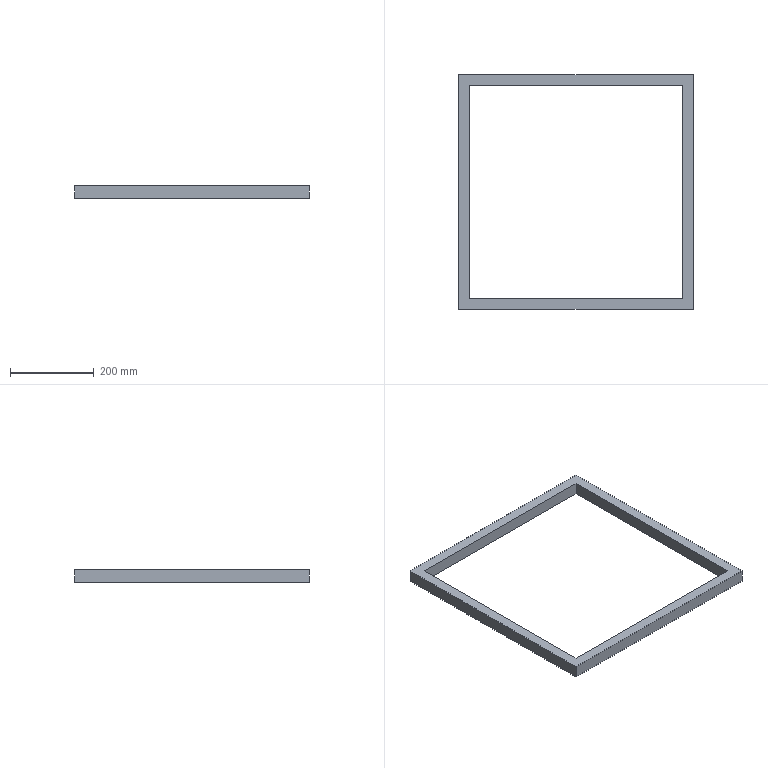Part | SolidWorks | features Extrusion 1 | 1 solid | 10 faces | box 560 x 560 x 30 mm | volume 1605000 mm3 | plane 10
STEP:
#1=CARTESIAN_POINT('',(0.,560.,30.));
#2=VERTEX_POINT('',#1);
#3=CARTESIAN_POINT('',(0.,0.,30.));
#4=VERTEX_POINT('',#3);
#5=CARTESIAN_POINT('',(0.,0.,30.));
#6=DIRECTION('',(0.,-1.,0.));
#7=VECTOR('',#6,1000.);
#8=LINE('',#5,#7);
#9=EDGE_CURVE('',#2,#4,#8,.T.);
#10=ORIENTED_EDGE('',*,*,#9,.T.);
#11=CARTESIAN_POINT('',(560.,0.,30.));
#12=VERTEX_POINT('',#11);
#13=CARTESIAN_POINT('',(0.,0.,30.));
#14=DIRECTION('',(1.,0.,0.));
#15=VECTOR('',#14,1000.);
#16=LINE('',#13,#15);
#17=EDGE_CURVE('',#4,#12,#16,.T.);
#18=ORIENTED_EDGE('',*,*,#17,.T.);
#19=CARTESIAN_POINT('',(560.,560.,30.));
#20=VERTEX_POINT('',#19);
#21=CARTESIAN_POINT('',(560.,0.,30.));
#22=DIRECTION('',(0.,1.,0.));
#23=VECTOR('',#22,1000.);
#24=LINE('',#21,#23);
#25=EDGE_CURVE('',#12,#20,#24,.T.);
#26=ORIENTED_EDGE('',*,*,#25,.T.);
#27=CARTESIAN_POINT('',(0.,560.,30.));
#28=DIRECTION('',(-1.,0.,0.));
#29=VECTOR('',#28,1000.);
#30=LINE('',#27,#29);
#31=EDGE_CURVE('',#20,#2,#30,.T.);
#32=ORIENTED_EDGE('',*,*,#31,.T.);
#33=EDGE_LOOP('',(#10,#18,#26,#32));
#34=FACE_OUTER_BOUND('',#33,.T.);
#35=CARTESIAN_POINT('',(25.,535.,30.));
#36=VERTEX_POINT('',#35);
#37=CARTESIAN_POINT('',(25.,25.,30.));
#38=VERTEX_POINT('',#37);
#39=CARTESIAN_POINT('',(25.,25.,30.));
#40=DIRECTION('',(0.,-1.,0.));
#41=VECTOR('',#40,1000.);
#42=LINE('',#39,#41);
#43=EDGE_CURVE('',#36,#38,#42,.T.);
#44=ORIENTED_EDGE('',*,*,#43,.F.);
#45=CARTESIAN_POINT('',(535.,535.,30.));
#46=VERTEX_POINT('',#45);
#47=CARTESIAN_POINT('',(25.,535.,30.));
#48=DIRECTION('',(-1.,0.,0.));
#49=VECTOR('',#48,1000.);
#50=LINE('',#47,#49);
#51=EDGE_CURVE('',#46,#36,#50,.T.);
#52=ORIENTED_EDGE('',*,*,#51,.F.);
#53=CARTESIAN_POINT('',(535.,25.,30.));
#54=VERTEX_POINT('',#53);
#55=CARTESIAN_POINT('',(535.,25.,30.));
#56=DIRECTION('',(0.,1.,0.));
#57=VECTOR('',#56,1000.);
#58=LINE('',#55,#57);
#59=EDGE_CURVE('',#54,#46,#58,.T.);
#60=ORIENTED_EDGE('',*,*,#59,.F.);
#61=CARTESIAN_POINT('',(25.,25.,30.));
#62=DIRECTION('',(1.,0.,0.));
#63=VECTOR('',#62,1000.);
#64=LINE('',#61,#63);
#65=EDGE_CURVE('',#38,#54,#64,.T.);
#66=ORIENTED_EDGE('',*,*,#65,.F.);
#67=EDGE_LOOP('',(#44,#52,#60,#66));
#68=FACE_BOUND('',#67,.T.);
#69=CARTESIAN_POINT('',(0.,0.,30.));
#70=DIRECTION('',(0.,0.,-1.));
#71=DIRECTION('',(-1.,0.,0.));
#72=AXIS2_PLACEMENT_3D('',#69,#70,#71);
#73=PLANE('',#72);
#74=ADVANCED_FACE('',(#34,#68),#73,.F.);
#75=CARTESIAN_POINT('',(0.,560.,0.));
#76=VERTEX_POINT('',#75);
#77=CARTESIAN_POINT('',(0.,0.,0.));
#78=VERTEX_POINT('',#77);
#79=CARTESIAN_POINT('',(0.,0.,0.));
#80=DIRECTION('',(0.,-1.,0.));
#81=VECTOR('',#80,1000.);
#82=LINE('',#79,#81);
#83=EDGE_CURVE('',#76,#78,#82,.T.);
#84=ORIENTED_EDGE('',*,*,#83,.F.);
#85=CARTESIAN_POINT('',(560.,560.,0.));
#86=VERTEX_POINT('',#85);
#87=CARTESIAN_POINT('',(0.,560.,0.));
#88=DIRECTION('',(-1.,0.,0.));
#89=VECTOR('',#88,1000.);
#90=LINE('',#87,#89);
#91=EDGE_CURVE('',#86,#76,#90,.T.);
#92=ORIENTED_EDGE('',*,*,#91,.F.);
#93=CARTESIAN_POINT('',(560.,0.,0.));
#94=VERTEX_POINT('',#93);
#95=CARTESIAN_POINT('',(560.,0.,0.));
#96=DIRECTION('',(0.,1.,0.));
#97=VECTOR('',#96,1000.);
#98=LINE('',#95,#97);
#99=EDGE_CURVE('',#94,#86,#98,.T.);
#100=ORIENTED_EDGE('',*,*,#99,.F.);
#101=CARTESIAN_POINT('',(0.,0.,0.));
#102=DIRECTION('',(1.,0.,0.));
#103=VECTOR('',#102,1000.);
#104=LINE('',#101,#103);
#105=EDGE_CURVE('',#78,#94,#104,.T.);
#106=ORIENTED_EDGE('',*,*,#105,.F.);
#107=EDGE_LOOP('',(#84,#92,#100,#106));
#108=FACE_OUTER_BOUND('',#107,.T.);
#109=CARTESIAN_POINT('',(535.,535.,0.));
#110=VERTEX_POINT('',#109);
#111=CARTESIAN_POINT('',(25.,535.,0.));
#112=VERTEX_POINT('',#111);
#113=CARTESIAN_POINT('',(25.,535.,0.));
#114=DIRECTION('',(-1.,0.,0.));
#115=VECTOR('',#114,1000.);
#116=LINE('',#113,#115);
#117=EDGE_CURVE('',#110,#112,#116,.T.);
#118=ORIENTED_EDGE('',*,*,#117,.T.);
#119=CARTESIAN_POINT('',(25.,25.,0.));
#120=VERTEX_POINT('',#119);
#121=CARTESIAN_POINT('',(25.,25.,0.));
#122=DIRECTION('',(0.,-1.,0.));
#123=VECTOR('',#122,1000.);
#124=LINE('',#121,#123);
#125=EDGE_CURVE('',#112,#120,#124,.T.);
#126=ORIENTED_EDGE('',*,*,#125,.T.);
#127=CARTESIAN_POINT('',(535.,25.,0.));
#128=VERTEX_POINT('',#127);
#129=CARTESIAN_POINT('',(25.,25.,0.));
#130=DIRECTION('',(1.,0.,0.));
#131=VECTOR('',#130,1000.);
#132=LINE('',#129,#131);
#133=EDGE_CURVE('',#120,#128,#132,.T.);
#134=ORIENTED_EDGE('',*,*,#133,.T.);
#135=CARTESIAN_POINT('',(535.,25.,0.));
#136=DIRECTION('',(0.,1.,0.));
#137=VECTOR('',#136,1000.);
#138=LINE('',#135,#137);
#139=EDGE_CURVE('',#128,#110,#138,.T.);
#140=ORIENTED_EDGE('',*,*,#139,.T.);
#141=EDGE_LOOP('',(#118,#126,#134,#140));
#142=FACE_BOUND('',#141,.T.);
#143=CARTESIAN_POINT('',(0.,0.,0.));
#144=DIRECTION('',(0.,0.,-1.));
#145=DIRECTION('',(-1.,0.,0.));
#146=AXIS2_PLACEMENT_3D('',#143,#144,#145);
#147=PLANE('',#146);
#148=ADVANCED_FACE('',(#108,#142),#147,.T.);
#149=ORIENTED_EDGE('',*,*,#83,.T.);
#150=CARTESIAN_POINT('',(0.,0.,30.));
#151=DIRECTION('',(0.,0.,-1.));
#152=VECTOR('',#151,1000.);
#153=LINE('',#150,#152);
#154=EDGE_CURVE('',#4,#78,#153,.T.);
#155=ORIENTED_EDGE('',*,*,#154,.F.);
#156=ORIENTED_EDGE('',*,*,#9,.F.);
#157=CARTESIAN_POINT('',(0.,560.,30.));
#158=DIRECTION('',(0.,0.,-1.));
#159=VECTOR('',#158,1000.);
#160=LINE('',#157,#159);
#161=EDGE_CURVE('',#2,#76,#160,.T.);
#162=ORIENTED_EDGE('',*,*,#161,.T.);
#163=EDGE_LOOP('',(#149,#155,#156,#162));
#164=FACE_OUTER_BOUND('',#163,.T.);
#165=CARTESIAN_POINT('',(0.,0.,30.));
#166=DIRECTION('',(1.,0.,0.));
#167=DIRECTION('',(0.,0.,-1.));
#168=AXIS2_PLACEMENT_3D('',#165,#166,#167);
#169=PLANE('',#168);
#170=ADVANCED_FACE('',(#164),#169,.F.);
#171=ORIENTED_EDGE('',*,*,#105,.T.);
#172=CARTESIAN_POINT('',(560.,0.,30.));
#173=DIRECTION('',(0.,0.,-1.));
#174=VECTOR('',#173,1000.);
#175=LINE('',#172,#174);
#176=EDGE_CURVE('',#12,#94,#175,.T.);
#177=ORIENTED_EDGE('',*,*,#176,.F.);
#178=ORIENTED_EDGE('',*,*,#17,.F.);
#179=ORIENTED_EDGE('',*,*,#154,.T.);
#180=EDGE_LOOP('',(#171,#177,#178,#179));
#181=FACE_OUTER_BOUND('',#180,.T.);
#182=CARTESIAN_POINT('',(0.,0.,30.));
#183=DIRECTION('',(0.,1.,0.));
#184=DIRECTION('',(0.,0.,1.));
#185=AXIS2_PLACEMENT_3D('',#182,#183,#184);
#186=PLANE('',#185);
#187=ADVANCED_FACE('',(#181),#186,.F.);
#188=ORIENTED_EDGE('',*,*,#99,.T.);
#189=CARTESIAN_POINT('',(560.,560.,30.));
#190=DIRECTION('',(0.,0.,-1.));
#191=VECTOR('',#190,1000.);
#192=LINE('',#189,#191);
#193=EDGE_CURVE('',#20,#86,#192,.T.);
#194=ORIENTED_EDGE('',*,*,#193,.F.);
#195=ORIENTED_EDGE('',*,*,#25,.F.);
#196=ORIENTED_EDGE('',*,*,#176,.T.);
#197=EDGE_LOOP('',(#188,#194,#195,#196));
#198=FACE_OUTER_BOUND('',#197,.T.);
#199=CARTESIAN_POINT('',(560.,0.,30.));
#200=DIRECTION('',(-1.,0.,0.));
#201=DIRECTION('',(0.,0.,1.));
#202=AXIS2_PLACEMENT_3D('',#199,#200,#201);
#203=PLANE('',#202);
#204=ADVANCED_FACE('',(#198),#203,.F.);
#205=ORIENTED_EDGE('',*,*,#91,.T.);
#206=ORIENTED_EDGE('',*,*,#161,.F.);
#207=ORIENTED_EDGE('',*,*,#31,.F.);
#208=ORIENTED_EDGE('',*,*,#193,.T.);
#209=EDGE_LOOP('',(#205,#206,#207,#208));
#210=FACE_OUTER_BOUND('',#209,.T.);
#211=CARTESIAN_POINT('',(0.,560.,30.));
#212=DIRECTION('',(0.,-1.,0.));
#213=DIRECTION('',(0.,0.,-1.));
#214=AXIS2_PLACEMENT_3D('',#211,#212,#213);
#215=PLANE('',#214);
#216=ADVANCED_FACE('',(#210),#215,.F.);
#217=ORIENTED_EDGE('',*,*,#125,.F.);
#218=CARTESIAN_POINT('',(25.,535.,30.));
#219=DIRECTION('',(0.,0.,-1.));
#220=VECTOR('',#219,1000.);
#221=LINE('',#218,#220);
#222=EDGE_CURVE('',#36,#112,#221,.T.);
#223=ORIENTED_EDGE('',*,*,#222,.F.);
#224=ORIENTED_EDGE('',*,*,#43,.T.);
#225=CARTESIAN_POINT('',(25.,25.,30.));
#226=DIRECTION('',(0.,0.,-1.));
#227=VECTOR('',#226,1000.);
#228=LINE('',#225,#227);
#229=EDGE_CURVE('',#38,#120,#228,.T.);
#230=ORIENTED_EDGE('',*,*,#229,.T.);
#231=EDGE_LOOP('',(#217,#223,#224,#230));
#232=FACE_OUTER_BOUND('',#231,.T.);
#233=CARTESIAN_POINT('',(25.,25.,30.));
#234=DIRECTION('',(1.,0.,0.));
#235=DIRECTION('',(0.,0.,-1.));
#236=AXIS2_PLACEMENT_3D('',#233,#234,#235);
#237=PLANE('',#236);
#238=ADVANCED_FACE('',(#232),#237,.T.);
#239=ORIENTED_EDGE('',*,*,#133,.F.);
#240=ORIENTED_EDGE('',*,*,#229,.F.);
#241=ORIENTED_EDGE('',*,*,#65,.T.);
#242=CARTESIAN_POINT('',(535.,25.,30.));
#243=DIRECTION('',(0.,0.,-1.));
#244=VECTOR('',#243,1000.);
#245=LINE('',#242,#244);
#246=EDGE_CURVE('',#54,#128,#245,.T.);
#247=ORIENTED_EDGE('',*,*,#246,.T.);
#248=EDGE_LOOP('',(#239,#240,#241,#247));
#249=FACE_OUTER_BOUND('',#248,.T.);
#250=CARTESIAN_POINT('',(25.,25.,30.));
#251=DIRECTION('',(0.,1.,0.));
#252=DIRECTION('',(0.,0.,1.));
#253=AXIS2_PLACEMENT_3D('',#250,#251,#252);
#254=PLANE('',#253);
#255=ADVANCED_FACE('',(#249),#254,.T.);
#256=ORIENTED_EDGE('',*,*,#139,.F.);
#257=ORIENTED_EDGE('',*,*,#246,.F.);
#258=ORIENTED_EDGE('',*,*,#59,.T.);
#259=CARTESIAN_POINT('',(535.,535.,30.));
#260=DIRECTION('',(0.,0.,-1.));
#261=VECTOR('',#260,1000.);
#262=LINE('',#259,#261);
#263=EDGE_CURVE('',#46,#110,#262,.T.);
#264=ORIENTED_EDGE('',*,*,#263,.T.);
#265=EDGE_LOOP('',(#256,#257,#258,#264));
#266=FACE_OUTER_BOUND('',#265,.T.);
#267=CARTESIAN_POINT('',(535.,25.,30.));
#268=DIRECTION('',(-1.,0.,0.));
#269=DIRECTION('',(0.,0.,1.));
#270=AXIS2_PLACEMENT_3D('',#267,#268,#269);
#271=PLANE('',#270);
#272=ADVANCED_FACE('',(#266),#271,.T.);
#273=ORIENTED_EDGE('',*,*,#117,.F.);
#274=ORIENTED_EDGE('',*,*,#263,.F.);
#275=ORIENTED_EDGE('',*,*,#51,.T.);
#276=ORIENTED_EDGE('',*,*,#222,.T.);
#277=EDGE_LOOP('',(#273,#274,#275,#276));
#278=FACE_OUTER_BOUND('',#277,.T.);
#279=CARTESIAN_POINT('',(25.,535.,30.));
#280=DIRECTION('',(0.,-1.,0.));
#281=DIRECTION('',(0.,0.,-1.));
#282=AXIS2_PLACEMENT_3D('',#279,#280,#281);
#283=PLANE('',#282);
#284=ADVANCED_FACE('',(#278),#283,.T.);
#285=CLOSED_SHELL('',(#74,#148,#170,#187,#204,#216,#238,#255,#272,#284));
#286=MANIFOLD_SOLID_BREP('',#285);
#287=CARTESIAN_POINT('',(0.,0.,0.));
#288=DIRECTION('',(0.,0.,1.));
#289=DIRECTION('',(1.,0.,0.));
#290=AXIS2_PLACEMENT_3D('',#287,#288,#289);
#291=(LENGTH_UNIT()NAMED_UNIT(*)SI_UNIT(.MILLI.,.METRE.));
#292=UNCERTAINTY_MEASURE_WITH_UNIT(LENGTH_MEASURE(0.00001),#291,'','');
#293=(NAMED_UNIT(*)PLANE_ANGLE_UNIT()SI_UNIT($,.RADIAN.));
#294=(NAMED_UNIT(*)SI_UNIT($,.STERADIAN.)SOLID_ANGLE_UNIT());
#295=(GEOMETRIC_REPRESENTATION_CONTEXT(3)GLOBAL_UNCERTAINTY_ASSIGNED_CONTEXT((#292))GLOBAL_UNIT_ASSIGNED_CONTEXT((#291,#293,#294))REPRESENTATION_CONTEXT('',''));
#296=ADVANCED_BREP_SHAPE_REPRESENTATION('',(#286,#290),#295);